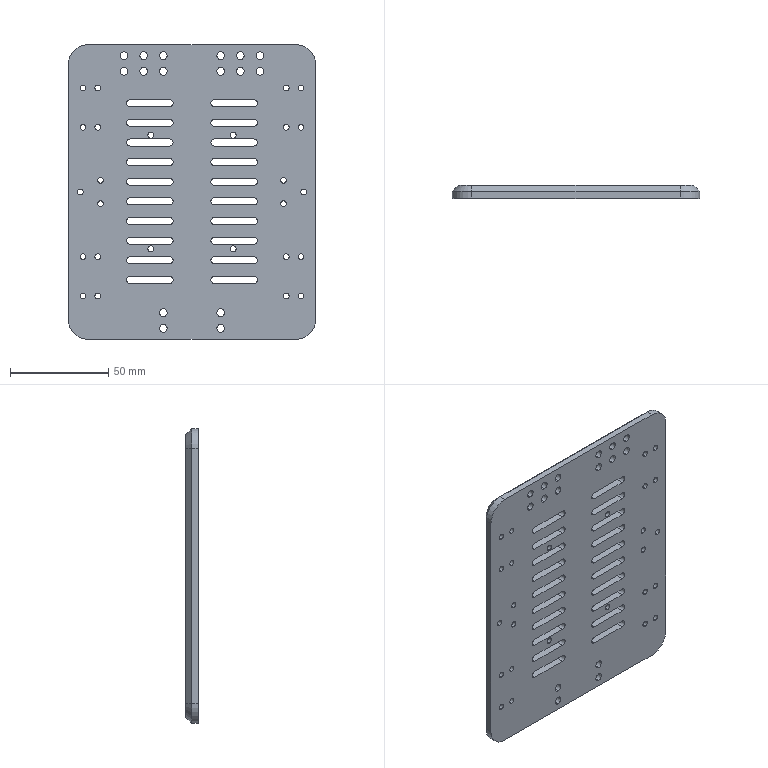Part | SolidWorks | features ICE 6, MirrorPattern 5, Chamfer 1, Extrusion 1, Fillet 1 | 1 solid | 182 faces | box 126 x 6.5 x 150 mm | volume 106751 mm3 | cylinder 128 | plane 50 | cone 4 | commonest cylinder face diameters 3 x52 3.593 x40 4 x32 20 x4